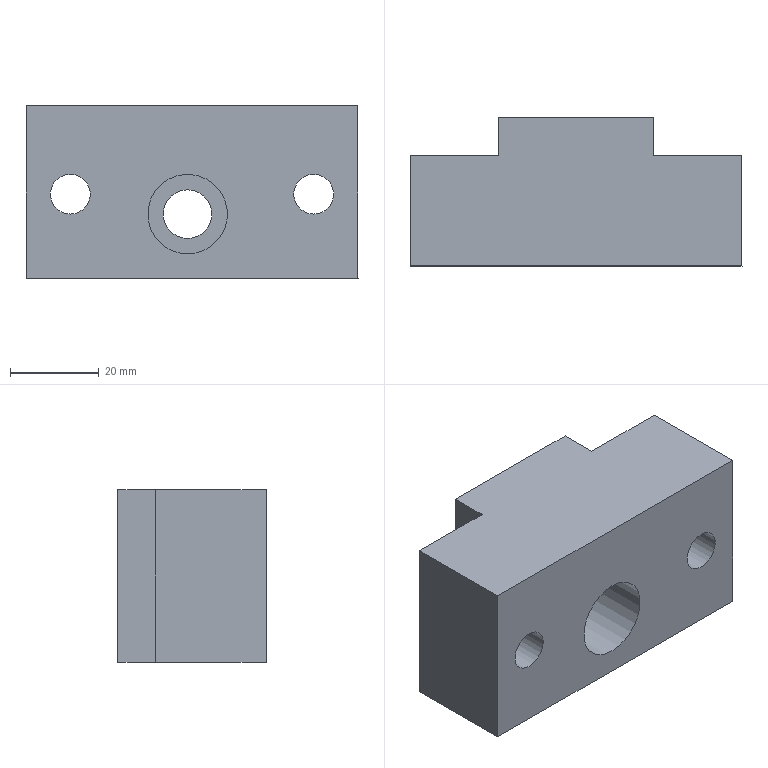Part | NX | features MAIN_BODY 2 | 1 solid | 15 faces | box 75 x 33.5 x 39 mm | volume 75413 mm3 | plane 11 | cylinder 4 | commonest cylinder face diameters 9 x2 11 x1 18 x1
STEP:
#1=CARTESIAN_POINT('',(-268.,-106.5,359.));
#2=VERTEX_POINT('',#1);
#3=CARTESIAN_POINT('',(-268.,-106.5,363.5));
#4=DIRECTION('',(0.,-1.,0.));
#5=DIRECTION('',(0.,0.,-1.));
#6=AXIS2_PLACEMENT_3D('',#3,#4,#5);
#7=CIRCLE('',#6,4.5);
#8=EDGE_CURVE('',#2,#2,#7,.F.);
#9=ORIENTED_EDGE('',*,*,#8,.T.);
#10=EDGE_LOOP('',(#9));
#11=FACE_BOUND('',#10,.T.);
#12=CARTESIAN_POINT('',(-323.,-106.5,359.));
#13=VERTEX_POINT('',#12);
#14=CARTESIAN_POINT('',(-323.,-106.5,363.5));
#15=DIRECTION('',(0.,-1.,0.));
#16=DIRECTION('',(0.,0.,-1.));
#17=AXIS2_PLACEMENT_3D('',#14,#15,#16);
#18=CIRCLE('',#17,4.5);
#19=EDGE_CURVE('',#13,#13,#18,.F.);
#20=ORIENTED_EDGE('',*,*,#19,.T.);
#21=EDGE_LOOP('',(#20));
#22=FACE_BOUND('',#21,.T.);
#23=CARTESIAN_POINT('',(-258.,-106.5,383.5));
#24=VERTEX_POINT('',#23);
#25=CARTESIAN_POINT('',(-258.,-106.5,344.5));
#26=VERTEX_POINT('',#25);
#27=CARTESIAN_POINT('',(-258.,-106.5,361.));
#28=DIRECTION('',(0.000000001,0.,-1.));
#29=VECTOR('',#28,1000.);
#30=LINE('',#27,#29);
#31=EDGE_CURVE('',#24,#26,#30,.T.);
#32=ORIENTED_EDGE('',*,*,#31,.F.);
#33=CARTESIAN_POINT('',(-333.,-106.5,383.5));
#34=VERTEX_POINT('',#33);
#35=CARTESIAN_POINT('',(-376.5,-106.5,383.5));
#36=DIRECTION('',(1.,0.,0.000000001));
#37=VECTOR('',#36,1000.);
#38=LINE('',#35,#37);
#39=EDGE_CURVE('',#34,#24,#38,.T.);
#40=ORIENTED_EDGE('',*,*,#39,.F.);
#41=CARTESIAN_POINT('',(-333.,-106.5,344.5));
#42=VERTEX_POINT('',#41);
#43=CARTESIAN_POINT('',(-333.,-106.5,361.));
#44=DIRECTION('',(-0.000000001,0.,1.));
#45=VECTOR('',#44,1000.);
#46=LINE('',#43,#45);
#47=EDGE_CURVE('',#42,#34,#46,.T.);
#48=ORIENTED_EDGE('',*,*,#47,.F.);
#49=CARTESIAN_POINT('',(-188.,-106.5,344.5));
#50=DIRECTION('',(1.,0.,0.000000001));
#51=VECTOR('',#50,1000.);
#52=LINE('',#49,#51);
#53=EDGE_CURVE('',#42,#26,#52,.T.);
#54=ORIENTED_EDGE('',*,*,#53,.T.);
#55=EDGE_LOOP('',(#32,#40,#48,#54));
#56=FACE_BOUND('',#55,.T.);
#57=CARTESIAN_POINT('',(-296.5,-106.5,350.));
#58=VERTEX_POINT('',#57);
#59=CARTESIAN_POINT('',(-296.5,-106.5,359.));
#60=DIRECTION('',(0.,-1.,0.));
#61=DIRECTION('',(0.,0.,-1.));
#62=AXIS2_PLACEMENT_3D('',#59,#60,#61);
#63=CIRCLE('',#62,9.);
#64=EDGE_CURVE('',#58,#58,#63,.T.);
#65=ORIENTED_EDGE('',*,*,#64,.F.);
#66=EDGE_LOOP('',(#65));
#67=FACE_BOUND('',#66,.T.);
#68=CARTESIAN_POINT('',(-570.,-106.5,380.));
#69=DIRECTION('',(0.,-1.,0.));
#70=DIRECTION('',(0.,0.,1.));
#71=AXIS2_PLACEMENT_3D('',#68,#69,#70);
#72=PLANE('',#71);
#73=ADVANCED_FACE('',(#11,#22,#56,#67),#72,.T.);
#74=CARTESIAN_POINT('',(-278.,-73.,344.5));
#75=VERTEX_POINT('',#74);
#76=CARTESIAN_POINT('',(-278.,-73.,383.5));
#77=VERTEX_POINT('',#76);
#78=CARTESIAN_POINT('',(-278.,-73.,359.));
#79=DIRECTION('',(0.000000001,-0.00000017,-1.));
#80=VECTOR('',#79,1000.);
#81=LINE('',#78,#80);
#82=EDGE_CURVE('',#75,#77,#81,.F.);
#83=ORIENTED_EDGE('',*,*,#82,.F.);
#84=CARTESIAN_POINT('',(-313.,-73.,344.5));
#85=VERTEX_POINT('',#84);
#86=CARTESIAN_POINT('',(-296.5,-73.,344.5));
#87=DIRECTION('',(-1.,-0.000000011,-0.000000001));
#88=VECTOR('',#87,1000.);
#89=LINE('',#86,#88);
#90=EDGE_CURVE('',#85,#75,#89,.F.);
#91=ORIENTED_EDGE('',*,*,#90,.F.);
#92=CARTESIAN_POINT('',(-313.,-73.,383.5));
#93=VERTEX_POINT('',#92);
#94=CARTESIAN_POINT('',(-313.,-73.,358.5));
#95=DIRECTION('',(-0.000000001,0.00000017,1.));
#96=VECTOR('',#95,1000.);
#97=LINE('',#94,#96);
#98=EDGE_CURVE('',#85,#93,#97,.T.);
#99=ORIENTED_EDGE('',*,*,#98,.T.);
#100=CARTESIAN_POINT('',(-296.5,-73.,383.5));
#101=DIRECTION('',(-1.,-0.000000011,-0.000000001));
#102=VECTOR('',#101,1000.);
#103=LINE('',#100,#102);
#104=EDGE_CURVE('',#93,#77,#103,.F.);
#105=ORIENTED_EDGE('',*,*,#104,.T.);
#106=EDGE_LOOP('',(#83,#91,#99,#105));
#107=FACE_BOUND('',#106,.T.);
#108=CARTESIAN_POINT('',(-296.5,-73.,353.5));
#109=VERTEX_POINT('',#108);
#110=CARTESIAN_POINT('',(-296.5,-73.,359.));
#111=DIRECTION('',(0.000000011,-1.,0.00000017));
#112=DIRECTION('',(0.,-0.00000017,-1.));
#113=AXIS2_PLACEMENT_3D('',#110,#111,#112);
#114=CIRCLE('',#113,5.5);
#115=EDGE_CURVE('',#109,#109,#114,.T.);
#116=ORIENTED_EDGE('',*,*,#115,.T.);
#117=EDGE_LOOP('',(#116));
#118=FACE_BOUND('',#117,.T.);
#119=CARTESIAN_POINT('',(-296.5,-73.,359.));
#120=DIRECTION('',(-0.000000011,1.,-0.00000017));
#121=DIRECTION('',(-0.000000001,0.00000017,1.));
#122=AXIS2_PLACEMENT_3D('',#119,#120,#121);
#123=PLANE('',#122);
#124=ADVANCED_FACE('',(#107,#118),#123,.T.);
#125=CARTESIAN_POINT('',(-323.,-81.5,359.));
#126=VERTEX_POINT('',#125);
#127=CARTESIAN_POINT('',(-323.,-81.5,363.5));
#128=DIRECTION('',(0.000000011,-1.,0.00000017));
#129=DIRECTION('',(0.,-0.00000017,-1.));
#130=AXIS2_PLACEMENT_3D('',#127,#128,#129);
#131=CIRCLE('',#130,4.5);
#132=EDGE_CURVE('',#126,#126,#131,.F.);
#133=ORIENTED_EDGE('',*,*,#132,.F.);
#134=EDGE_LOOP('',(#133));
#135=FACE_BOUND('',#134,.T.);
#136=CARTESIAN_POINT('',(-313.,-81.5,383.5));
#137=VERTEX_POINT('',#136);
#138=CARTESIAN_POINT('',(-313.,-81.5,344.5));
#139=VERTEX_POINT('',#138);
#140=CARTESIAN_POINT('',(-313.,-81.5,358.5));
#141=DIRECTION('',(-0.000000001,0.00000017,1.));
#142=VECTOR('',#141,1000.);
#143=LINE('',#140,#142);
#144=EDGE_CURVE('',#137,#139,#143,.F.);
#145=ORIENTED_EDGE('',*,*,#144,.T.);
#146=CARTESIAN_POINT('',(-333.,-81.5,344.5));
#147=VERTEX_POINT('',#146);
#148=CARTESIAN_POINT('',(-188.,-81.5,344.5));
#149=DIRECTION('',(1.,0.000000011,0.000000001));
#150=VECTOR('',#149,1000.);
#151=LINE('',#148,#150);
#152=EDGE_CURVE('',#147,#139,#151,.T.);
#153=ORIENTED_EDGE('',*,*,#152,.F.);
#154=CARTESIAN_POINT('',(-333.,-81.5,383.5));
#155=VERTEX_POINT('',#154);
#156=CARTESIAN_POINT('',(-333.,-81.5,361.));
#157=DIRECTION('',(-0.000000001,0.00000017,1.));
#158=VECTOR('',#157,1000.);
#159=LINE('',#156,#158);
#160=EDGE_CURVE('',#147,#155,#159,.T.);
#161=ORIENTED_EDGE('',*,*,#160,.T.);
#162=CARTESIAN_POINT('',(-376.5,-81.5,383.5));
#163=DIRECTION('',(1.,0.000000011,0.000000001));
#164=VECTOR('',#163,1000.);
#165=LINE('',#162,#164);
#166=EDGE_CURVE('',#155,#137,#165,.T.);
#167=ORIENTED_EDGE('',*,*,#166,.T.);
#168=EDGE_LOOP('',(#145,#153,#161,#167));
#169=FACE_BOUND('',#168,.T.);
#170=CARTESIAN_POINT('',(-313.,-81.5,361.));
#171=DIRECTION('',(0.000000011,-1.,0.00000017));
#172=DIRECTION('',(0.000000001,-0.00000017,-1.));
#173=AXIS2_PLACEMENT_3D('',#170,#171,#172);
#174=PLANE('',#173);
#175=ADVANCED_FACE('',(#135,#169),#174,.F.);
#176=CARTESIAN_POINT('',(-268.,-81.5,359.));
#177=VERTEX_POINT('',#176);
#178=CARTESIAN_POINT('',(-268.,-81.5,363.5));
#179=DIRECTION('',(0.000000011,-1.,0.00000017));
#180=DIRECTION('',(0.,-0.00000017,-1.));
#181=AXIS2_PLACEMENT_3D('',#178,#179,#180);
#182=CIRCLE('',#181,4.5);
#183=EDGE_CURVE('',#177,#177,#182,.F.);
#184=ORIENTED_EDGE('',*,*,#183,.F.);
#185=EDGE_LOOP('',(#184));
#186=FACE_BOUND('',#185,.T.);
#187=CARTESIAN_POINT('',(-278.,-81.5,344.5));
#188=VERTEX_POINT('',#187);
#189=CARTESIAN_POINT('',(-278.,-81.5,383.5));
#190=VERTEX_POINT('',#189);
#191=CARTESIAN_POINT('',(-278.,-81.5,358.5));
#192=DIRECTION('',(-0.000000001,0.00000017,1.));
#193=VECTOR('',#192,1000.);
#194=LINE('',#191,#193);
#195=EDGE_CURVE('',#188,#190,#194,.T.);
#196=ORIENTED_EDGE('',*,*,#195,.T.);
#197=CARTESIAN_POINT('',(-258.,-81.5,383.5));
#198=VERTEX_POINT('',#197);
#199=CARTESIAN_POINT('',(-376.5,-81.5,383.5));
#200=DIRECTION('',(1.,0.000000011,0.000000001));
#201=VECTOR('',#200,1000.);
#202=LINE('',#199,#201);
#203=EDGE_CURVE('',#190,#198,#202,.T.);
#204=ORIENTED_EDGE('',*,*,#203,.T.);
#205=CARTESIAN_POINT('',(-258.,-81.5,344.5));
#206=VERTEX_POINT('',#205);
#207=CARTESIAN_POINT('',(-258.,-81.5,361.));
#208=DIRECTION('',(0.000000001,-0.00000017,-1.));
#209=VECTOR('',#208,1000.);
#210=LINE('',#207,#209);
#211=EDGE_CURVE('',#198,#206,#210,.T.);
#212=ORIENTED_EDGE('',*,*,#211,.T.);
#213=CARTESIAN_POINT('',(-188.,-81.5,344.5));
#214=DIRECTION('',(1.,0.000000011,0.000000001));
#215=VECTOR('',#214,1000.);
#216=LINE('',#213,#215);
#217=EDGE_CURVE('',#188,#206,#216,.T.);
#218=ORIENTED_EDGE('',*,*,#217,.F.);
#219=EDGE_LOOP('',(#196,#204,#212,#218));
#220=FACE_BOUND('',#219,.T.);
#221=CARTESIAN_POINT('',(-313.,-81.5,361.));
#222=DIRECTION('',(0.000000011,-1.,0.00000017));
#223=DIRECTION('',(0.000000001,-0.00000017,-1.));
#224=AXIS2_PLACEMENT_3D('',#221,#222,#223);
#225=PLANE('',#224);
#226=ADVANCED_FACE('',(#186,#220),#225,.F.);
#227=CARTESIAN_POINT('',(-278.,-92.,383.5));
#228=DIRECTION('',(-0.000000011,1.,-0.00000017));
#229=VECTOR('',#228,1000.);
#230=LINE('',#227,#229);
#231=EDGE_CURVE('',#77,#190,#230,.F.);
#232=ORIENTED_EDGE('',*,*,#231,.F.);
#233=ORIENTED_EDGE('',*,*,#104,.F.);
#234=CARTESIAN_POINT('',(-313.,-92.,383.5));
#235=DIRECTION('',(0.000000011,-1.,0.00000017));
#236=VECTOR('',#235,1000.);
#237=LINE('',#234,#236);
#238=EDGE_CURVE('',#93,#137,#237,.T.);
#239=ORIENTED_EDGE('',*,*,#238,.T.);
#240=ORIENTED_EDGE('',*,*,#166,.F.);
#241=CARTESIAN_POINT('',(-333.,-92.,383.5));
#242=DIRECTION('',(0.000000011,-1.,0.00000017));
#243=VECTOR('',#242,1000.);
#244=LINE('',#241,#243);
#245=EDGE_CURVE('',#155,#34,#244,.T.);
#246=ORIENTED_EDGE('',*,*,#245,.T.);
#247=ORIENTED_EDGE('',*,*,#39,.T.);
#248=CARTESIAN_POINT('',(-258.,-92.,383.5));
#249=DIRECTION('',(0.000000011,-1.,0.00000017));
#250=VECTOR('',#249,1000.);
#251=LINE('',#248,#250);
#252=EDGE_CURVE('',#198,#24,#251,.T.);
#253=ORIENTED_EDGE('',*,*,#252,.F.);
#254=ORIENTED_EDGE('',*,*,#203,.F.);
#255=EDGE_LOOP('',(#232,#233,#239,#240,#246,#247,#253,#254));
#256=FACE_BOUND('',#255,.T.);
#257=CARTESIAN_POINT('',(-376.5,-92.,383.5));
#258=DIRECTION('',(-0.000000001,0.00000017,1.));
#259=DIRECTION('',(1.,0.000000011,0.000000001));
#260=AXIS2_PLACEMENT_3D('',#257,#258,#259);
#261=PLANE('',#260);
#262=ADVANCED_FACE('',(#256),#261,.T.);
#263=ORIENTED_EDGE('',*,*,#47,.T.);
#264=ORIENTED_EDGE('',*,*,#245,.F.);
#265=ORIENTED_EDGE('',*,*,#160,.F.);
#266=CARTESIAN_POINT('',(-333.,-92.,344.5));
#267=DIRECTION('',(0.000000011,-1.,0.00000017));
#268=VECTOR('',#267,1000.);
#269=LINE('',#266,#268);
#270=EDGE_CURVE('',#147,#42,#269,.T.);
#271=ORIENTED_EDGE('',*,*,#270,.T.);
#272=EDGE_LOOP('',(#263,#264,#265,#271));
#273=FACE_BOUND('',#272,.T.);
#274=CARTESIAN_POINT('',(-333.,-92.,361.));
#275=DIRECTION('',(-1.,-0.000000011,-0.000000001));
#276=DIRECTION('',(-0.000000001,0.00000017,1.));
#277=AXIS2_PLACEMENT_3D('',#274,#275,#276);
#278=PLANE('',#277);
#279=ADVANCED_FACE('',(#273),#278,.T.);
#280=ORIENTED_EDGE('',*,*,#217,.T.);
#281=CARTESIAN_POINT('',(-258.,-103.,344.5));
#282=DIRECTION('',(0.000000011,-1.,0.00000017));
#283=VECTOR('',#282,1000.);
#284=LINE('',#281,#283);
#285=EDGE_CURVE('',#206,#26,#284,.T.);
#286=ORIENTED_EDGE('',*,*,#285,.T.);
#287=ORIENTED_EDGE('',*,*,#53,.F.);
#288=ORIENTED_EDGE('',*,*,#270,.F.);
#289=ORIENTED_EDGE('',*,*,#152,.T.);
#290=CARTESIAN_POINT('',(-313.,-103.,344.5));
#291=DIRECTION('',(-0.000000011,1.,-0.00000017));
#292=VECTOR('',#291,1000.);
#293=LINE('',#290,#292);
#294=EDGE_CURVE('',#85,#139,#293,.F.);
#295=ORIENTED_EDGE('',*,*,#294,.F.);
#296=ORIENTED_EDGE('',*,*,#90,.T.);
#297=CARTESIAN_POINT('',(-278.,-92.,344.5));
#298=DIRECTION('',(0.000000011,-1.,0.00000017));
#299=VECTOR('',#298,1000.);
#300=LINE('',#297,#299);
#301=EDGE_CURVE('',#75,#188,#300,.T.);
#302=ORIENTED_EDGE('',*,*,#301,.T.);
#303=EDGE_LOOP('',(#280,#286,#287,#288,#289,#295,#296,#302));
#304=FACE_BOUND('',#303,.T.);
#305=CARTESIAN_POINT('',(-188.,-103.,344.5));
#306=DIRECTION('',(-0.000000001,0.00000017,1.));
#307=DIRECTION('',(1.,0.000000011,0.000000001));
#308=AXIS2_PLACEMENT_3D('',#305,#306,#307);
#309=PLANE('',#308);
#310=ADVANCED_FACE('',(#304),#309,.F.);
#311=ORIENTED_EDGE('',*,*,#31,.T.);
#312=ORIENTED_EDGE('',*,*,#285,.F.);
#313=ORIENTED_EDGE('',*,*,#211,.F.);
#314=ORIENTED_EDGE('',*,*,#252,.T.);
#315=EDGE_LOOP('',(#311,#312,#313,#314));
#316=FACE_BOUND('',#315,.T.);
#317=CARTESIAN_POINT('',(-258.,-92.,361.));
#318=DIRECTION('',(1.,0.000000011,0.000000001));
#319=DIRECTION('',(0.000000001,-0.00000017,-1.));
#320=AXIS2_PLACEMENT_3D('',#317,#318,#319);
#321=PLANE('',#320);
#322=ADVANCED_FACE('',(#316),#321,.T.);
#323=ORIENTED_EDGE('',*,*,#238,.F.);
#324=ORIENTED_EDGE('',*,*,#98,.F.);
#325=ORIENTED_EDGE('',*,*,#294,.T.);
#326=ORIENTED_EDGE('',*,*,#144,.F.);
#327=EDGE_LOOP('',(#323,#324,#325,#326));
#328=FACE_BOUND('',#327,.T.);
#329=CARTESIAN_POINT('',(-313.,-92.,358.5));
#330=DIRECTION('',(-1.,-0.000000011,-0.000000001));
#331=DIRECTION('',(-0.000000001,0.00000017,1.));
#332=AXIS2_PLACEMENT_3D('',#329,#330,#331);
#333=PLANE('',#332);
#334=ADVANCED_FACE('',(#328),#333,.T.);
#335=ORIENTED_EDGE('',*,*,#301,.F.);
#336=ORIENTED_EDGE('',*,*,#82,.T.);
#337=ORIENTED_EDGE('',*,*,#231,.T.);
#338=ORIENTED_EDGE('',*,*,#195,.F.);
#339=EDGE_LOOP('',(#335,#336,#337,#338));
#340=FACE_BOUND('',#339,.T.);
#341=CARTESIAN_POINT('',(-278.,-92.,358.5));
#342=DIRECTION('',(-1.,-0.000000011,-0.000000001));
#343=DIRECTION('',(-0.000000001,0.00000017,1.));
#344=AXIS2_PLACEMENT_3D('',#341,#342,#343);
#345=PLANE('',#344);
#346=ADVANCED_FACE('',(#340),#345,.F.);
#347=ORIENTED_EDGE('',*,*,#19,.F.);
#348=EDGE_LOOP('',(#347));
#349=FACE_BOUND('',#348,.T.);
#350=ORIENTED_EDGE('',*,*,#132,.T.);
#351=EDGE_LOOP('',(#350));
#352=FACE_BOUND('',#351,.T.);
#353=CARTESIAN_POINT('',(-323.,-92.,363.5));
#354=DIRECTION('',(0.000000011,-1.,0.00000017));
#355=DIRECTION('',(-0.000000001,0.00000017,1.));
#356=AXIS2_PLACEMENT_3D('',#353,#354,#355);
#357=CYLINDRICAL_SURFACE('',#356,4.5);
#358=ADVANCED_FACE('',(#349,#352),#357,.F.);
#359=ORIENTED_EDGE('',*,*,#8,.F.);
#360=EDGE_LOOP('',(#359));
#361=FACE_BOUND('',#360,.T.);
#362=ORIENTED_EDGE('',*,*,#183,.T.);
#363=EDGE_LOOP('',(#362));
#364=FACE_BOUND('',#363,.T.);
#365=CARTESIAN_POINT('',(-268.,-92.,363.5));
#366=DIRECTION('',(0.000000011,-1.,0.00000017));
#367=DIRECTION('',(-0.000000001,0.00000017,1.));
#368=AXIS2_PLACEMENT_3D('',#365,#366,#367);
#369=CYLINDRICAL_SURFACE('',#368,4.5);
#370=ADVANCED_FACE('',(#361,#364),#369,.F.);
#371=CARTESIAN_POINT('',(-296.5,-88.,353.5));
#372=VERTEX_POINT('',#371);
#373=CARTESIAN_POINT('',(-296.5,-88.,359.));
#374=DIRECTION('',(0.000000011,-1.,0.00000017));
#375=DIRECTION('',(0.,-0.00000017,-1.));
#376=AXIS2_PLACEMENT_3D('',#373,#374,#375);
#377=CIRCLE('',#376,5.5);
#378=EDGE_CURVE('',#372,#372,#377,.T.);
#379=ORIENTED_EDGE('',*,*,#378,.T.);
#380=EDGE_LOOP('',(#379));
#381=FACE_BOUND('',#380,.T.);
#382=ORIENTED_EDGE('',*,*,#115,.F.);
#383=EDGE_LOOP('',(#382));
#384=FACE_BOUND('',#383,.T.);
#385=CARTESIAN_POINT('',(-296.5,-73.,359.));
#386=DIRECTION('',(0.000000011,-1.,0.00000017));
#387=DIRECTION('',(0.,0.00000017,1.));
#388=AXIS2_PLACEMENT_3D('',#385,#386,#387);
#389=CYLINDRICAL_SURFACE('',#388,5.5);
#390=ADVANCED_FACE('',(#381,#384),#389,.F.);
#391=CARTESIAN_POINT('',(-296.5,-88.,350.));
#392=VERTEX_POINT('',#391);
#393=CARTESIAN_POINT('',(-296.5,-88.,359.));
#394=DIRECTION('',(0.000000011,-1.,0.00000017));
#395=DIRECTION('',(0.,-0.00000017,-1.));
#396=AXIS2_PLACEMENT_3D('',#393,#394,#395);
#397=CIRCLE('',#396,9.);
#398=EDGE_CURVE('',#392,#392,#397,.T.);
#399=ORIENTED_EDGE('',*,*,#398,.T.);
#400=EDGE_LOOP('',(#399));
#401=FACE_BOUND('',#400,.T.);
#402=ORIENTED_EDGE('',*,*,#378,.F.);
#403=EDGE_LOOP('',(#402));
#404=FACE_BOUND('',#403,.T.);
#405=CARTESIAN_POINT('',(-296.5,-88.,359.));
#406=DIRECTION('',(0.000000011,-1.,0.00000017));
#407=DIRECTION('',(0.,0.00000017,1.));
#408=AXIS2_PLACEMENT_3D('',#405,#406,#407);
#409=PLANE('',#408);
#410=ADVANCED_FACE('',(#401,#404),#409,.T.);
#411=ORIENTED_EDGE('',*,*,#64,.T.);
#412=EDGE_LOOP('',(#411));
#413=FACE_BOUND('',#412,.T.);
#414=ORIENTED_EDGE('',*,*,#398,.F.);
#415=EDGE_LOOP('',(#414));
#416=FACE_BOUND('',#415,.T.);
#417=CARTESIAN_POINT('',(-296.5,-86.,359.));
#418=DIRECTION('',(0.000000011,-1.,0.00000017));
#419=DIRECTION('',(0.,0.00000017,1.));
#420=AXIS2_PLACEMENT_3D('',#417,#418,#419);
#421=CYLINDRICAL_SURFACE('',#420,9.);
#422=ADVANCED_FACE('',(#413,#416),#421,.F.);
#423=CLOSED_SHELL('',(#73,#124,#175,#226,#262,#279,#310,#322,#334,#346,#358,#370,#390,#410,#422));
#424=MANIFOLD_SOLID_BREP('',#423);
#425=(LENGTH_UNIT()NAMED_UNIT(*)SI_UNIT(.MILLI.,.METRE.));
#426=UNCERTAINTY_MEASURE_WITH_UNIT(LENGTH_MEASURE(0.00001),#425,'','');
#427=(NAMED_UNIT(*)PLANE_ANGLE_UNIT()SI_UNIT($,.RADIAN.));
#428=(NAMED_UNIT(*)SI_UNIT($,.STERADIAN.)SOLID_ANGLE_UNIT());
#429=(GEOMETRIC_REPRESENTATION_CONTEXT(3)GLOBAL_UNCERTAINTY_ASSIGNED_CONTEXT((#426))GLOBAL_UNIT_ASSIGNED_CONTEXT((#425,#427,#428))REPRESENTATION_CONTEXT('',''));
#430=ADVANCED_BREP_SHAPE_REPRESENTATION('',(#424),#429);